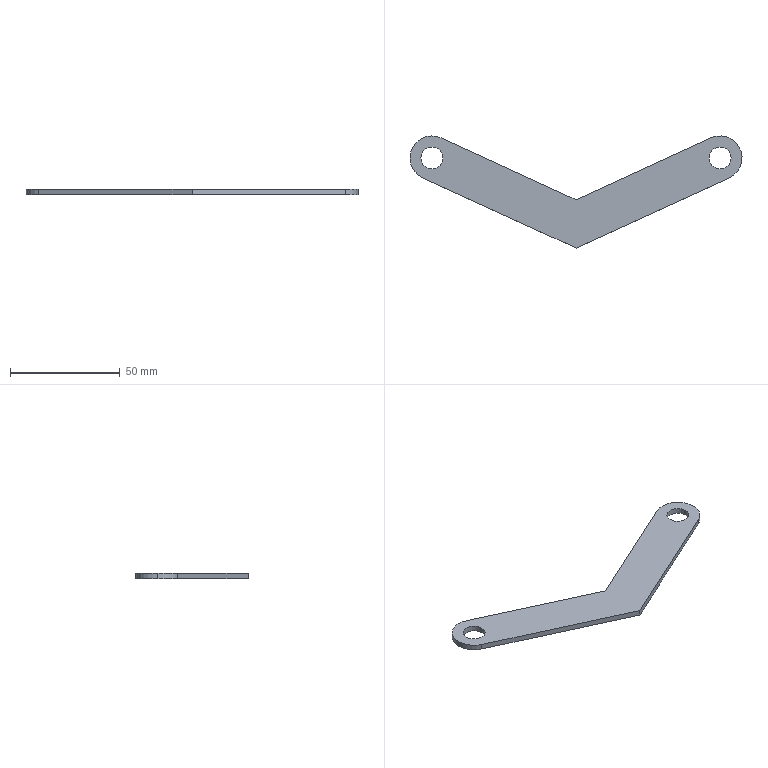Part | SolidWorks | features Extrusion 1 | 1 solid | 13 faces | box 151.1 x 51.002 x 2.5 mm | volume 7602 mm3 | cylinder 7 | plane 6 | commonest cylinder face diameters 10 x4 20 x3
STEP:
#1=CARTESIAN_POINT('',(60.55,41.002,2.5));
#2=VERTEX_POINT('',#1);
#3=CARTESIAN_POINT('',(70.55,41.002,2.5));
#4=VERTEX_POINT('',#3);
#5=CARTESIAN_POINT('',(65.55,41.002,2.5));
#6=DIRECTION('',(0.,0.,1.));
#7=DIRECTION('',(1.,0.,0.));
#8=AXIS2_PLACEMENT_3D('',#5,#6,#7);
#9=CIRCLE('',#8,5.);
#10=EDGE_CURVE('',#2,#4,#9,.T.);
#11=ORIENTED_EDGE('',*,*,#10,.T.);
#12=CARTESIAN_POINT('',(70.55,41.002,0.));
#13=VERTEX_POINT('',#12);
#14=CARTESIAN_POINT('',(70.55,41.002,2.5));
#15=DIRECTION('',(0.,0.,-1.));
#16=VECTOR('',#15,1000.);
#17=LINE('',#14,#16);
#18=EDGE_CURVE('',#4,#13,#17,.T.);
#19=ORIENTED_EDGE('',*,*,#18,.T.);
#20=CARTESIAN_POINT('',(60.55,41.002,0.));
#21=VERTEX_POINT('',#20);
#22=CARTESIAN_POINT('',(65.55,41.002,0.));
#23=DIRECTION('',(0.,0.,1.));
#24=DIRECTION('',(1.,0.,0.));
#25=AXIS2_PLACEMENT_3D('',#22,#23,#24);
#26=CIRCLE('',#25,5.);
#27=EDGE_CURVE('',#21,#13,#26,.T.);
#28=ORIENTED_EDGE('',*,*,#27,.F.);
#29=CARTESIAN_POINT('',(60.55,41.002,2.5));
#30=DIRECTION('',(0.,0.,-1.));
#31=VECTOR('',#30,1000.);
#32=LINE('',#29,#31);
#33=EDGE_CURVE('',#2,#21,#32,.T.);
#34=ORIENTED_EDGE('',*,*,#33,.F.);
#35=EDGE_LOOP('',(#11,#19,#28,#34));
#36=FACE_OUTER_BOUND('',#35,.T.);
#37=CARTESIAN_POINT('',(65.55,41.002,2.5));
#38=DIRECTION('',(0.,0.,-1.));
#39=DIRECTION('',(-1.,0.,0.));
#40=AXIS2_PLACEMENT_3D('',#37,#38,#39);
#41=CYLINDRICAL_SURFACE('',#40,5.);
#42=ADVANCED_FACE('',(#36),#41,.F.);
#43=CARTESIAN_POINT('',(-70.55,41.002,2.5));
#44=VERTEX_POINT('',#43);
#45=CARTESIAN_POINT('',(-60.55,41.002,2.5));
#46=VERTEX_POINT('',#45);
#47=CARTESIAN_POINT('',(-65.55,41.002,2.5));
#48=DIRECTION('',(0.,0.,1.));
#49=DIRECTION('',(1.,0.,0.));
#50=AXIS2_PLACEMENT_3D('',#47,#48,#49);
#51=CIRCLE('',#50,5.);
#52=EDGE_CURVE('',#44,#46,#51,.T.);
#53=ORIENTED_EDGE('',*,*,#52,.T.);
#54=CARTESIAN_POINT('',(-60.55,41.002,0.));
#55=VERTEX_POINT('',#54);
#56=CARTESIAN_POINT('',(-60.55,41.002,2.5));
#57=DIRECTION('',(0.,0.,-1.));
#58=VECTOR('',#57,1000.);
#59=LINE('',#56,#58);
#60=EDGE_CURVE('',#46,#55,#59,.T.);
#61=ORIENTED_EDGE('',*,*,#60,.T.);
#62=CARTESIAN_POINT('',(-70.55,41.002,0.));
#63=VERTEX_POINT('',#62);
#64=CARTESIAN_POINT('',(-65.55,41.002,0.));
#65=DIRECTION('',(0.,0.,1.));
#66=DIRECTION('',(1.,0.,0.));
#67=AXIS2_PLACEMENT_3D('',#64,#65,#66);
#68=CIRCLE('',#67,5.);
#69=EDGE_CURVE('',#63,#55,#68,.T.);
#70=ORIENTED_EDGE('',*,*,#69,.F.);
#71=CARTESIAN_POINT('',(-70.55,41.002,2.5));
#72=DIRECTION('',(0.,0.,-1.));
#73=VECTOR('',#72,1000.);
#74=LINE('',#71,#73);
#75=EDGE_CURVE('',#44,#63,#74,.T.);
#76=ORIENTED_EDGE('',*,*,#75,.F.);
#77=EDGE_LOOP('',(#53,#61,#70,#76));
#78=FACE_OUTER_BOUND('',#77,.T.);
#79=CARTESIAN_POINT('',(-65.55,41.002,2.5));
#80=DIRECTION('',(0.,0.,-1.));
#81=DIRECTION('',(-1.,0.,0.));
#82=AXIS2_PLACEMENT_3D('',#79,#80,#81);
#83=CYLINDRICAL_SURFACE('',#82,5.);
#84=ADVANCED_FACE('',(#78),#83,.F.);
#85=CARTESIAN_POINT('',(-75.55,41.002,2.5));
#86=VERTEX_POINT('',#85);
#87=CARTESIAN_POINT('',(-69.712,31.909,2.5));
#88=VERTEX_POINT('',#87);
#89=CARTESIAN_POINT('',(-65.55,41.002,2.5));
#90=DIRECTION('',(0.,0.,1.));
#91=DIRECTION('',(-1.,0.,0.));
#92=AXIS2_PLACEMENT_3D('',#89,#90,#91);
#93=CIRCLE('',#92,10.);
#94=EDGE_CURVE('',#86,#88,#93,.T.);
#95=ORIENTED_EDGE('',*,*,#94,.F.);
#96=CARTESIAN_POINT('',(-75.55,41.002,0.));
#97=VERTEX_POINT('',#96);
#98=CARTESIAN_POINT('',(-75.55,41.002,2.5));
#99=DIRECTION('',(0.,0.,-1.));
#100=VECTOR('',#99,1000.);
#101=LINE('',#98,#100);
#102=EDGE_CURVE('',#86,#97,#101,.T.);
#103=ORIENTED_EDGE('',*,*,#102,.T.);
#104=CARTESIAN_POINT('',(-69.712,31.909,0.));
#105=VERTEX_POINT('',#104);
#106=CARTESIAN_POINT('',(-65.55,41.002,0.));
#107=DIRECTION('',(0.,0.,1.));
#108=DIRECTION('',(-1.,0.,0.));
#109=AXIS2_PLACEMENT_3D('',#106,#107,#108);
#110=CIRCLE('',#109,10.);
#111=EDGE_CURVE('',#97,#105,#110,.T.);
#112=ORIENTED_EDGE('',*,*,#111,.T.);
#113=CARTESIAN_POINT('',(-69.712,31.909,2.5));
#114=DIRECTION('',(0.,0.,-1.));
#115=VECTOR('',#114,1000.);
#116=LINE('',#113,#115);
#117=EDGE_CURVE('',#88,#105,#116,.T.);
#118=ORIENTED_EDGE('',*,*,#117,.F.);
#119=EDGE_LOOP('',(#95,#103,#112,#118));
#120=FACE_OUTER_BOUND('',#119,.T.);
#121=CARTESIAN_POINT('',(-65.55,41.002,2.5));
#122=DIRECTION('',(0.,0.,-1.));
#123=DIRECTION('',(-1.,0.,0.));
#124=AXIS2_PLACEMENT_3D('',#121,#122,#123);
#125=CYLINDRICAL_SURFACE('',#124,10.);
#126=ADVANCED_FACE('',(#120),#125,.T.);
#127=CARTESIAN_POINT('',(0.,0.,2.5));
#128=VERTEX_POINT('',#127);
#129=CARTESIAN_POINT('',(0.,0.,2.5));
#130=DIRECTION('',(0.9093,-0.4162,0.));
#131=VECTOR('',#130,1000.);
#132=LINE('',#129,#131);
#133=EDGE_CURVE('',#88,#128,#132,.T.);
#134=ORIENTED_EDGE('',*,*,#133,.T.);
#135=CARTESIAN_POINT('',(69.712,31.909,2.5));
#136=VERTEX_POINT('',#135);
#137=CARTESIAN_POINT('',(0.,0.,2.5));
#138=DIRECTION('',(0.9093,0.4162,0.));
#139=VECTOR('',#138,1000.);
#140=LINE('',#137,#139);
#141=EDGE_CURVE('',#128,#136,#140,.T.);
#142=ORIENTED_EDGE('',*,*,#141,.T.);
#143=CARTESIAN_POINT('',(61.388,50.095,2.5));
#144=VERTEX_POINT('',#143);
#145=CARTESIAN_POINT('',(65.55,41.002,2.5));
#146=DIRECTION('',(0.,0.,1.));
#147=DIRECTION('',(1.,0.,0.));
#148=AXIS2_PLACEMENT_3D('',#145,#146,#147);
#149=CIRCLE('',#148,10.);
#150=EDGE_CURVE('',#136,#144,#149,.T.);
#151=ORIENTED_EDGE('',*,*,#150,.T.);
#152=CARTESIAN_POINT('',(0.,21.996,2.5));
#153=VERTEX_POINT('',#152);
#154=CARTESIAN_POINT('',(0.,21.996,2.5));
#155=DIRECTION('',(-0.9093,-0.4162,0.));
#156=VECTOR('',#155,1000.);
#157=LINE('',#154,#156);
#158=EDGE_CURVE('',#144,#153,#157,.T.);
#159=ORIENTED_EDGE('',*,*,#158,.T.);
#160=CARTESIAN_POINT('',(-61.388,50.095,2.5));
#161=VERTEX_POINT('',#160);
#162=CARTESIAN_POINT('',(0.,21.996,2.5));
#163=DIRECTION('',(-0.9093,0.4162,0.));
#164=VECTOR('',#163,1000.);
#165=LINE('',#162,#164);
#166=EDGE_CURVE('',#153,#161,#165,.T.);
#167=ORIENTED_EDGE('',*,*,#166,.T.);
#168=CARTESIAN_POINT('',(-65.55,41.002,2.5));
#169=DIRECTION('',(0.,0.,1.));
#170=DIRECTION('',(-1.,0.,0.));
#171=AXIS2_PLACEMENT_3D('',#168,#169,#170);
#172=CIRCLE('',#171,10.);
#173=EDGE_CURVE('',#161,#86,#172,.T.);
#174=ORIENTED_EDGE('',*,*,#173,.T.);
#175=ORIENTED_EDGE('',*,*,#94,.T.);
#176=EDGE_LOOP('',(#134,#142,#151,#159,#167,#174,#175));
#177=FACE_OUTER_BOUND('',#176,.T.);
#178=ORIENTED_EDGE('',*,*,#52,.F.);
#179=CARTESIAN_POINT('',(-65.55,41.002,2.5));
#180=DIRECTION('',(0.,0.,1.));
#181=DIRECTION('',(1.,0.,0.));
#182=AXIS2_PLACEMENT_3D('',#179,#180,#181);
#183=CIRCLE('',#182,5.);
#184=EDGE_CURVE('',#46,#44,#183,.T.);
#185=ORIENTED_EDGE('',*,*,#184,.F.);
#186=EDGE_LOOP('',(#178,#185));
#187=FACE_BOUND('',#186,.T.);
#188=ORIENTED_EDGE('',*,*,#10,.F.);
#189=CARTESIAN_POINT('',(65.55,41.002,2.5));
#190=DIRECTION('',(0.,0.,1.));
#191=DIRECTION('',(1.,0.,0.));
#192=AXIS2_PLACEMENT_3D('',#189,#190,#191);
#193=CIRCLE('',#192,5.);
#194=EDGE_CURVE('',#4,#2,#193,.T.);
#195=ORIENTED_EDGE('',*,*,#194,.F.);
#196=EDGE_LOOP('',(#188,#195));
#197=FACE_BOUND('',#196,.T.);
#198=CARTESIAN_POINT('',(-65.55,41.002,2.5));
#199=DIRECTION('',(0.,0.,-1.));
#200=DIRECTION('',(-1.,0.,0.));
#201=AXIS2_PLACEMENT_3D('',#198,#199,#200);
#202=PLANE('',#201);
#203=ADVANCED_FACE('',(#177,#187,#197),#202,.F.);
#204=ORIENTED_EDGE('',*,*,#69,.T.);
#205=CARTESIAN_POINT('',(-65.55,41.002,0.));
#206=DIRECTION('',(0.,0.,1.));
#207=DIRECTION('',(1.,0.,0.));
#208=AXIS2_PLACEMENT_3D('',#205,#206,#207);
#209=CIRCLE('',#208,5.);
#210=EDGE_CURVE('',#55,#63,#209,.T.);
#211=ORIENTED_EDGE('',*,*,#210,.T.);
#212=EDGE_LOOP('',(#204,#211));
#213=FACE_BOUND('',#212,.T.);
#214=CARTESIAN_POINT('',(0.,0.,0.));
#215=VERTEX_POINT('',#214);
#216=CARTESIAN_POINT('',(0.,0.,0.));
#217=DIRECTION('',(0.9093,-0.4162,0.));
#218=VECTOR('',#217,1000.);
#219=LINE('',#216,#218);
#220=EDGE_CURVE('',#105,#215,#219,.T.);
#221=ORIENTED_EDGE('',*,*,#220,.F.);
#222=ORIENTED_EDGE('',*,*,#111,.F.);
#223=CARTESIAN_POINT('',(-61.388,50.095,0.));
#224=VERTEX_POINT('',#223);
#225=CARTESIAN_POINT('',(-65.55,41.002,0.));
#226=DIRECTION('',(0.,0.,1.));
#227=DIRECTION('',(-1.,0.,0.));
#228=AXIS2_PLACEMENT_3D('',#225,#226,#227);
#229=CIRCLE('',#228,10.);
#230=EDGE_CURVE('',#224,#97,#229,.T.);
#231=ORIENTED_EDGE('',*,*,#230,.F.);
#232=CARTESIAN_POINT('',(0.,21.996,0.));
#233=VERTEX_POINT('',#232);
#234=CARTESIAN_POINT('',(0.,21.996,0.));
#235=DIRECTION('',(-0.9093,0.4162,0.));
#236=VECTOR('',#235,1000.);
#237=LINE('',#234,#236);
#238=EDGE_CURVE('',#233,#224,#237,.T.);
#239=ORIENTED_EDGE('',*,*,#238,.F.);
#240=CARTESIAN_POINT('',(61.388,50.095,0.));
#241=VERTEX_POINT('',#240);
#242=CARTESIAN_POINT('',(0.,21.996,0.));
#243=DIRECTION('',(-0.9093,-0.4162,0.));
#244=VECTOR('',#243,1000.);
#245=LINE('',#242,#244);
#246=EDGE_CURVE('',#241,#233,#245,.T.);
#247=ORIENTED_EDGE('',*,*,#246,.F.);
#248=CARTESIAN_POINT('',(69.712,31.909,0.));
#249=VERTEX_POINT('',#248);
#250=CARTESIAN_POINT('',(65.55,41.002,0.));
#251=DIRECTION('',(0.,0.,1.));
#252=DIRECTION('',(1.,0.,0.));
#253=AXIS2_PLACEMENT_3D('',#250,#251,#252);
#254=CIRCLE('',#253,10.);
#255=EDGE_CURVE('',#249,#241,#254,.T.);
#256=ORIENTED_EDGE('',*,*,#255,.F.);
#257=CARTESIAN_POINT('',(0.,0.,0.));
#258=DIRECTION('',(0.9093,0.4162,0.));
#259=VECTOR('',#258,1000.);
#260=LINE('',#257,#259);
#261=EDGE_CURVE('',#215,#249,#260,.T.);
#262=ORIENTED_EDGE('',*,*,#261,.F.);
#263=EDGE_LOOP('',(#221,#222,#231,#239,#247,#256,#262));
#264=FACE_OUTER_BOUND('',#263,.T.);
#265=ORIENTED_EDGE('',*,*,#27,.T.);
#266=CARTESIAN_POINT('',(65.55,41.002,0.));
#267=DIRECTION('',(0.,0.,1.));
#268=DIRECTION('',(1.,0.,0.));
#269=AXIS2_PLACEMENT_3D('',#266,#267,#268);
#270=CIRCLE('',#269,5.);
#271=EDGE_CURVE('',#13,#21,#270,.T.);
#272=ORIENTED_EDGE('',*,*,#271,.T.);
#273=EDGE_LOOP('',(#265,#272));
#274=FACE_BOUND('',#273,.T.);
#275=CARTESIAN_POINT('',(-65.55,41.002,0.));
#276=DIRECTION('',(0.,0.,-1.));
#277=DIRECTION('',(-1.,0.,0.));
#278=AXIS2_PLACEMENT_3D('',#275,#276,#277);
#279=PLANE('',#278);
#280=ADVANCED_FACE('',(#213,#264,#274),#279,.T.);
#281=ORIENTED_EDGE('',*,*,#220,.T.);
#282=CARTESIAN_POINT('',(0.,0.,2.5));
#283=DIRECTION('',(0.,0.,-1.));
#284=VECTOR('',#283,1000.);
#285=LINE('',#282,#284);
#286=EDGE_CURVE('',#128,#215,#285,.T.);
#287=ORIENTED_EDGE('',*,*,#286,.F.);
#288=ORIENTED_EDGE('',*,*,#133,.F.);
#289=ORIENTED_EDGE('',*,*,#117,.T.);
#290=EDGE_LOOP('',(#281,#287,#288,#289));
#291=FACE_OUTER_BOUND('',#290,.T.);
#292=CARTESIAN_POINT('',(0.,0.,2.5));
#293=DIRECTION('',(0.4162,0.9093,0.));
#294=DIRECTION('',(-0.9093,0.4162,0.));
#295=AXIS2_PLACEMENT_3D('',#292,#293,#294);
#296=PLANE('',#295);
#297=ADVANCED_FACE('',(#291),#296,.F.);
#298=ORIENTED_EDGE('',*,*,#261,.T.);
#299=CARTESIAN_POINT('',(69.712,31.909,2.5));
#300=DIRECTION('',(0.,0.,-1.));
#301=VECTOR('',#300,1000.);
#302=LINE('',#299,#301);
#303=EDGE_CURVE('',#136,#249,#302,.T.);
#304=ORIENTED_EDGE('',*,*,#303,.F.);
#305=ORIENTED_EDGE('',*,*,#141,.F.);
#306=ORIENTED_EDGE('',*,*,#286,.T.);
#307=EDGE_LOOP('',(#298,#304,#305,#306));
#308=FACE_OUTER_BOUND('',#307,.T.);
#309=CARTESIAN_POINT('',(0.,0.,2.5));
#310=DIRECTION('',(-0.4162,0.9093,0.));
#311=DIRECTION('',(-0.9093,-0.4162,0.));
#312=AXIS2_PLACEMENT_3D('',#309,#310,#311);
#313=PLANE('',#312);
#314=ADVANCED_FACE('',(#308),#313,.F.);
#315=ORIENTED_EDGE('',*,*,#255,.T.);
#316=CARTESIAN_POINT('',(61.388,50.095,2.5));
#317=DIRECTION('',(0.,0.,-1.));
#318=VECTOR('',#317,1000.);
#319=LINE('',#316,#318);
#320=EDGE_CURVE('',#144,#241,#319,.T.);
#321=ORIENTED_EDGE('',*,*,#320,.F.);
#322=ORIENTED_EDGE('',*,*,#150,.F.);
#323=ORIENTED_EDGE('',*,*,#303,.T.);
#324=EDGE_LOOP('',(#315,#321,#322,#323));
#325=FACE_OUTER_BOUND('',#324,.T.);
#326=CARTESIAN_POINT('',(65.55,41.002,2.5));
#327=DIRECTION('',(0.,0.,-1.));
#328=DIRECTION('',(-1.,0.,0.));
#329=AXIS2_PLACEMENT_3D('',#326,#327,#328);
#330=CYLINDRICAL_SURFACE('',#329,10.);
#331=ADVANCED_FACE('',(#325),#330,.T.);
#332=ORIENTED_EDGE('',*,*,#246,.T.);
#333=CARTESIAN_POINT('',(0.,21.996,2.5));
#334=DIRECTION('',(0.,0.,-1.));
#335=VECTOR('',#334,1000.);
#336=LINE('',#333,#335);
#337=EDGE_CURVE('',#153,#233,#336,.T.);
#338=ORIENTED_EDGE('',*,*,#337,.F.);
#339=ORIENTED_EDGE('',*,*,#158,.F.);
#340=ORIENTED_EDGE('',*,*,#320,.T.);
#341=EDGE_LOOP('',(#332,#338,#339,#340));
#342=FACE_OUTER_BOUND('',#341,.T.);
#343=CARTESIAN_POINT('',(0.,21.996,2.5));
#344=DIRECTION('',(0.4162,-0.9093,0.));
#345=DIRECTION('',(0.9093,0.4162,0.));
#346=AXIS2_PLACEMENT_3D('',#343,#344,#345);
#347=PLANE('',#346);
#348=ADVANCED_FACE('',(#342),#347,.F.);
#349=ORIENTED_EDGE('',*,*,#238,.T.);
#350=CARTESIAN_POINT('',(-61.388,50.095,2.5));
#351=DIRECTION('',(0.,0.,-1.));
#352=VECTOR('',#351,1000.);
#353=LINE('',#350,#352);
#354=EDGE_CURVE('',#161,#224,#353,.T.);
#355=ORIENTED_EDGE('',*,*,#354,.F.);
#356=ORIENTED_EDGE('',*,*,#166,.F.);
#357=ORIENTED_EDGE('',*,*,#337,.T.);
#358=EDGE_LOOP('',(#349,#355,#356,#357));
#359=FACE_OUTER_BOUND('',#358,.T.);
#360=CARTESIAN_POINT('',(0.,21.996,2.5));
#361=DIRECTION('',(-0.4162,-0.9093,0.));
#362=DIRECTION('',(0.9093,-0.4162,0.));
#363=AXIS2_PLACEMENT_3D('',#360,#361,#362);
#364=PLANE('',#363);
#365=ADVANCED_FACE('',(#359),#364,.F.);
#366=ORIENTED_EDGE('',*,*,#102,.F.);
#367=ORIENTED_EDGE('',*,*,#173,.F.);
#368=ORIENTED_EDGE('',*,*,#354,.T.);
#369=ORIENTED_EDGE('',*,*,#230,.T.);
#370=EDGE_LOOP('',(#366,#367,#368,#369));
#371=FACE_OUTER_BOUND('',#370,.T.);
#372=CARTESIAN_POINT('',(-65.55,41.002,2.5));
#373=DIRECTION('',(0.,0.,-1.));
#374=DIRECTION('',(-1.,0.,0.));
#375=AXIS2_PLACEMENT_3D('',#372,#373,#374);
#376=CYLINDRICAL_SURFACE('',#375,10.);
#377=ADVANCED_FACE('',(#371),#376,.T.);
#378=ORIENTED_EDGE('',*,*,#60,.F.);
#379=ORIENTED_EDGE('',*,*,#184,.T.);
#380=ORIENTED_EDGE('',*,*,#75,.T.);
#381=ORIENTED_EDGE('',*,*,#210,.F.);
#382=EDGE_LOOP('',(#378,#379,#380,#381));
#383=FACE_OUTER_BOUND('',#382,.T.);
#384=CARTESIAN_POINT('',(-65.55,41.002,2.5));
#385=DIRECTION('',(0.,0.,-1.));
#386=DIRECTION('',(-1.,0.,0.));
#387=AXIS2_PLACEMENT_3D('',#384,#385,#386);
#388=CYLINDRICAL_SURFACE('',#387,5.);
#389=ADVANCED_FACE('',(#383),#388,.F.);
#390=ORIENTED_EDGE('',*,*,#18,.F.);
#391=ORIENTED_EDGE('',*,*,#194,.T.);
#392=ORIENTED_EDGE('',*,*,#33,.T.);
#393=ORIENTED_EDGE('',*,*,#271,.F.);
#394=EDGE_LOOP('',(#390,#391,#392,#393));
#395=FACE_OUTER_BOUND('',#394,.T.);
#396=CARTESIAN_POINT('',(65.55,41.002,2.5));
#397=DIRECTION('',(0.,0.,-1.));
#398=DIRECTION('',(-1.,0.,0.));
#399=AXIS2_PLACEMENT_3D('',#396,#397,#398);
#400=CYLINDRICAL_SURFACE('',#399,5.);
#401=ADVANCED_FACE('',(#395),#400,.F.);
#402=CLOSED_SHELL('',(#42,#84,#126,#203,#280,#297,#314,#331,#348,#365,#377,#389,#401));
#403=MANIFOLD_SOLID_BREP('',#402);
#404=CARTESIAN_POINT('',(0.,0.,0.));
#405=DIRECTION('',(0.,0.,1.));
#406=DIRECTION('',(1.,0.,0.));
#407=AXIS2_PLACEMENT_3D('',#404,#405,#406);
#408=(LENGTH_UNIT()NAMED_UNIT(*)SI_UNIT(.MILLI.,.METRE.));
#409=UNCERTAINTY_MEASURE_WITH_UNIT(LENGTH_MEASURE(0.00001),#408,'','');
#410=(NAMED_UNIT(*)PLANE_ANGLE_UNIT()SI_UNIT($,.RADIAN.));
#411=(NAMED_UNIT(*)SI_UNIT($,.STERADIAN.)SOLID_ANGLE_UNIT());
#412=(GEOMETRIC_REPRESENTATION_CONTEXT(3)GLOBAL_UNCERTAINTY_ASSIGNED_CONTEXT((#409))GLOBAL_UNIT_ASSIGNED_CONTEXT((#408,#410,#411))REPRESENTATION_CONTEXT('',''));
#413=ADVANCED_BREP_SHAPE_REPRESENTATION('',(#403,#407),#412);